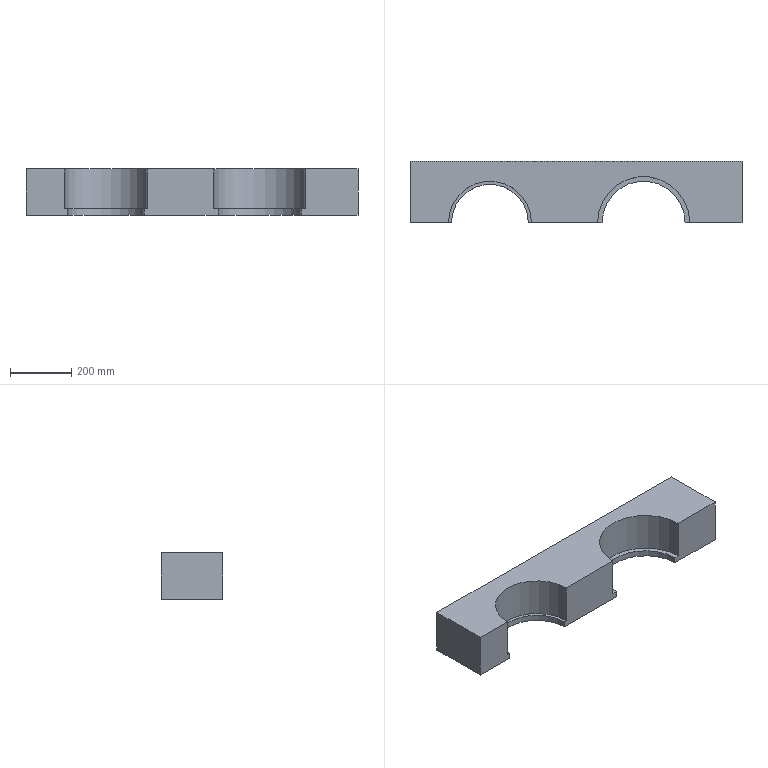Part | SolidWorks | features ICE 2, RefAxis 2, Extrusion 1 | 1 solid | 14 faces | box 1080 x 200 x 150 mm | volume 23020382 mm3 | plane 10 | cylinder 4 | commonest cylinder face diameters 270 x2 250 x1 300 x1
STEP:
#1=CARTESIAN_POINT('',(-540.,-100.,0.));
#2=VERTEX_POINT('',#1);
#3=CARTESIAN_POINT('',(-405.,-100.,0.));
#4=VERTEX_POINT('',#3);
#5=CARTESIAN_POINT('',(540.,-100.,0.));
#6=DIRECTION('',(1.,0.,0.));
#7=VECTOR('',#6,1000.);
#8=LINE('',#5,#7);
#9=EDGE_CURVE('',#2,#4,#8,.T.);
#10=ORIENTED_EDGE('',*,*,#9,.T.);
#11=CARTESIAN_POINT('',(-405.,-100.,20.));
#12=VERTEX_POINT('',#11);
#13=CARTESIAN_POINT('',(-405.,-100.,0.));
#14=DIRECTION('',(0.,0.,1.));
#15=VECTOR('',#14,1000.);
#16=LINE('',#13,#15);
#17=EDGE_CURVE('',#4,#12,#16,.T.);
#18=ORIENTED_EDGE('',*,*,#17,.T.);
#19=CARTESIAN_POINT('',(-415.,-100.,20.));
#20=VERTEX_POINT('',#19);
#21=CARTESIAN_POINT('',(540.,-100.,20.));
#22=DIRECTION('',(1.,0.,0.));
#23=VECTOR('',#22,1000.);
#24=LINE('',#21,#23);
#25=EDGE_CURVE('',#20,#12,#24,.T.);
#26=ORIENTED_EDGE('',*,*,#25,.F.);
#27=CARTESIAN_POINT('',(-415.,-100.,150.));
#28=VERTEX_POINT('',#27);
#29=CARTESIAN_POINT('',(-415.,-100.,20.));
#30=DIRECTION('',(0.,0.,1.));
#31=VECTOR('',#30,1000.);
#32=LINE('',#29,#31);
#33=EDGE_CURVE('',#20,#28,#32,.T.);
#34=ORIENTED_EDGE('',*,*,#33,.T.);
#35=CARTESIAN_POINT('',(-540.,-100.,150.));
#36=VERTEX_POINT('',#35);
#37=CARTESIAN_POINT('',(540.,-100.,150.));
#38=DIRECTION('',(1.,0.,0.));
#39=VECTOR('',#38,1000.);
#40=LINE('',#37,#39);
#41=EDGE_CURVE('',#36,#28,#40,.T.);
#42=ORIENTED_EDGE('',*,*,#41,.F.);
#43=CARTESIAN_POINT('',(-540.,-100.,150.));
#44=DIRECTION('',(0.,0.,-1.));
#45=VECTOR('',#44,1000.);
#46=LINE('',#43,#45);
#47=EDGE_CURVE('',#36,#2,#46,.T.);
#48=ORIENTED_EDGE('',*,*,#47,.T.);
#49=EDGE_LOOP('',(#10,#18,#26,#34,#42,#48));
#50=FACE_OUTER_BOUND('',#49,.T.);
#51=CARTESIAN_POINT('',(540.,-100.,150.));
#52=DIRECTION('',(0.,1.,0.));
#53=DIRECTION('',(-1.,0.,0.));
#54=AXIS2_PLACEMENT_3D('',#51,#52,#53);
#55=PLANE('',#54);
#56=ADVANCED_FACE('',(#50),#55,.F.);
#57=CARTESIAN_POINT('',(-155.,-100.,20.));
#58=VERTEX_POINT('',#57);
#59=CARTESIAN_POINT('',(-145.,-100.,20.));
#60=VERTEX_POINT('',#59);
#61=CARTESIAN_POINT('',(540.,-100.,20.));
#62=DIRECTION('',(1.,0.,0.));
#63=VECTOR('',#62,1000.);
#64=LINE('',#61,#63);
#65=EDGE_CURVE('',#58,#60,#64,.T.);
#66=ORIENTED_EDGE('',*,*,#65,.F.);
#67=CARTESIAN_POINT('',(-155.,-100.,0.));
#68=VERTEX_POINT('',#67);
#69=CARTESIAN_POINT('',(-155.,-100.,0.));
#70=DIRECTION('',(0.,0.,-1.));
#71=VECTOR('',#70,1000.);
#72=LINE('',#69,#71);
#73=EDGE_CURVE('',#58,#68,#72,.T.);
#74=ORIENTED_EDGE('',*,*,#73,.T.);
#75=CARTESIAN_POINT('',(85.,-100.,0.));
#76=VERTEX_POINT('',#75);
#77=CARTESIAN_POINT('',(540.,-100.,0.));
#78=DIRECTION('',(1.,0.,0.));
#79=VECTOR('',#78,1000.);
#80=LINE('',#77,#79);
#81=EDGE_CURVE('',#68,#76,#80,.T.);
#82=ORIENTED_EDGE('',*,*,#81,.T.);
#83=CARTESIAN_POINT('',(85.,-100.,20.));
#84=VERTEX_POINT('',#83);
#85=CARTESIAN_POINT('',(85.,-100.,0.));
#86=DIRECTION('',(0.,0.,1.));
#87=VECTOR('',#86,1000.);
#88=LINE('',#85,#87);
#89=EDGE_CURVE('',#76,#84,#88,.T.);
#90=ORIENTED_EDGE('',*,*,#89,.T.);
#91=CARTESIAN_POINT('',(70.,-100.,20.));
#92=VERTEX_POINT('',#91);
#93=CARTESIAN_POINT('',(540.,-100.,20.));
#94=DIRECTION('',(1.,0.,0.));
#95=VECTOR('',#94,1000.);
#96=LINE('',#93,#95);
#97=EDGE_CURVE('',#92,#84,#96,.T.);
#98=ORIENTED_EDGE('',*,*,#97,.F.);
#99=CARTESIAN_POINT('',(70.,-100.,150.));
#100=VERTEX_POINT('',#99);
#101=CARTESIAN_POINT('',(70.,-100.,20.));
#102=DIRECTION('',(0.,0.,1.));
#103=VECTOR('',#102,1000.);
#104=LINE('',#101,#103);
#105=EDGE_CURVE('',#92,#100,#104,.T.);
#106=ORIENTED_EDGE('',*,*,#105,.T.);
#107=CARTESIAN_POINT('',(-145.,-100.,150.));
#108=VERTEX_POINT('',#107);
#109=CARTESIAN_POINT('',(540.,-100.,150.));
#110=DIRECTION('',(1.,0.,0.));
#111=VECTOR('',#110,1000.);
#112=LINE('',#109,#111);
#113=EDGE_CURVE('',#108,#100,#112,.T.);
#114=ORIENTED_EDGE('',*,*,#113,.F.);
#115=CARTESIAN_POINT('',(-145.,-100.,20.));
#116=DIRECTION('',(0.,0.,-1.));
#117=VECTOR('',#116,1000.);
#118=LINE('',#115,#117);
#119=EDGE_CURVE('',#108,#60,#118,.T.);
#120=ORIENTED_EDGE('',*,*,#119,.T.);
#121=EDGE_LOOP('',(#66,#74,#82,#90,#98,#106,#114,#120));
#122=FACE_OUTER_BOUND('',#121,.T.);
#123=CARTESIAN_POINT('',(540.,-100.,150.));
#124=DIRECTION('',(0.,1.,0.));
#125=DIRECTION('',(-1.,0.,0.));
#126=AXIS2_PLACEMENT_3D('',#123,#124,#125);
#127=PLANE('',#126);
#128=ADVANCED_FACE('',(#122),#127,.F.);
#129=CARTESIAN_POINT('',(-540.,100.,0.));
#130=VERTEX_POINT('',#129);
#131=CARTESIAN_POINT('',(-540.,100.,0.));
#132=DIRECTION('',(0.,-1.,0.));
#133=VECTOR('',#132,1000.);
#134=LINE('',#131,#133);
#135=EDGE_CURVE('',#130,#2,#134,.T.);
#136=ORIENTED_EDGE('',*,*,#135,.T.);
#137=ORIENTED_EDGE('',*,*,#47,.F.);
#138=CARTESIAN_POINT('',(-540.,100.,150.));
#139=VERTEX_POINT('',#138);
#140=CARTESIAN_POINT('',(-540.,100.,150.));
#141=DIRECTION('',(0.,-1.,0.));
#142=VECTOR('',#141,1000.);
#143=LINE('',#140,#142);
#144=EDGE_CURVE('',#139,#36,#143,.T.);
#145=ORIENTED_EDGE('',*,*,#144,.F.);
#146=CARTESIAN_POINT('',(-540.,100.,150.));
#147=DIRECTION('',(0.,0.,-1.));
#148=VECTOR('',#147,1000.);
#149=LINE('',#146,#148);
#150=EDGE_CURVE('',#139,#130,#149,.T.);
#151=ORIENTED_EDGE('',*,*,#150,.T.);
#152=EDGE_LOOP('',(#136,#137,#145,#151));
#153=FACE_OUTER_BOUND('',#152,.T.);
#154=CARTESIAN_POINT('',(-540.,100.,150.));
#155=DIRECTION('',(1.,0.,0.));
#156=DIRECTION('',(0.,0.,-1.));
#157=AXIS2_PLACEMENT_3D('',#154,#155,#156);
#158=PLANE('',#157);
#159=ADVANCED_FACE('',(#153),#158,.F.);
#160=CARTESIAN_POINT('',(355.,-100.,20.));
#161=VERTEX_POINT('',#160);
#162=CARTESIAN_POINT('',(370.,-100.,20.));
#163=VERTEX_POINT('',#162);
#164=CARTESIAN_POINT('',(540.,-100.,20.));
#165=DIRECTION('',(1.,0.,0.));
#166=VECTOR('',#165,1000.);
#167=LINE('',#164,#166);
#168=EDGE_CURVE('',#161,#163,#167,.T.);
#169=ORIENTED_EDGE('',*,*,#168,.F.);
#170=CARTESIAN_POINT('',(355.,-100.,0.));
#171=VERTEX_POINT('',#170);
#172=CARTESIAN_POINT('',(355.,-100.,0.));
#173=DIRECTION('',(0.,0.,-1.));
#174=VECTOR('',#173,1000.);
#175=LINE('',#172,#174);
#176=EDGE_CURVE('',#161,#171,#175,.T.);
#177=ORIENTED_EDGE('',*,*,#176,.T.);
#178=CARTESIAN_POINT('',(540.,-100.,0.));
#179=VERTEX_POINT('',#178);
#180=CARTESIAN_POINT('',(540.,-100.,0.));
#181=DIRECTION('',(1.,0.,0.));
#182=VECTOR('',#181,1000.);
#183=LINE('',#180,#182);
#184=EDGE_CURVE('',#171,#179,#183,.T.);
#185=ORIENTED_EDGE('',*,*,#184,.T.);
#186=CARTESIAN_POINT('',(540.,-100.,150.));
#187=VERTEX_POINT('',#186);
#188=CARTESIAN_POINT('',(540.,-100.,150.));
#189=DIRECTION('',(0.,0.,-1.));
#190=VECTOR('',#189,1000.);
#191=LINE('',#188,#190);
#192=EDGE_CURVE('',#187,#179,#191,.T.);
#193=ORIENTED_EDGE('',*,*,#192,.F.);
#194=CARTESIAN_POINT('',(370.,-100.,150.));
#195=VERTEX_POINT('',#194);
#196=CARTESIAN_POINT('',(540.,-100.,150.));
#197=DIRECTION('',(1.,0.,0.));
#198=VECTOR('',#197,1000.);
#199=LINE('',#196,#198);
#200=EDGE_CURVE('',#195,#187,#199,.T.);
#201=ORIENTED_EDGE('',*,*,#200,.F.);
#202=CARTESIAN_POINT('',(370.,-100.,20.));
#203=DIRECTION('',(0.,0.,-1.));
#204=VECTOR('',#203,1000.);
#205=LINE('',#202,#204);
#206=EDGE_CURVE('',#195,#163,#205,.T.);
#207=ORIENTED_EDGE('',*,*,#206,.T.);
#208=EDGE_LOOP('',(#169,#177,#185,#193,#201,#207));
#209=FACE_OUTER_BOUND('',#208,.T.);
#210=CARTESIAN_POINT('',(540.,-100.,150.));
#211=DIRECTION('',(0.,1.,0.));
#212=DIRECTION('',(-1.,0.,0.));
#213=AXIS2_PLACEMENT_3D('',#210,#211,#212);
#214=PLANE('',#213);
#215=ADVANCED_FACE('',(#209),#214,.F.);
#216=CARTESIAN_POINT('',(540.,100.,0.));
#217=VERTEX_POINT('',#216);
#218=CARTESIAN_POINT('',(540.,100.,0.));
#219=DIRECTION('',(0.,1.,0.));
#220=VECTOR('',#219,1000.);
#221=LINE('',#218,#220);
#222=EDGE_CURVE('',#179,#217,#221,.T.);
#223=ORIENTED_EDGE('',*,*,#222,.T.);
#224=CARTESIAN_POINT('',(540.,100.,150.));
#225=VERTEX_POINT('',#224);
#226=CARTESIAN_POINT('',(540.,100.,150.));
#227=DIRECTION('',(0.,0.,-1.));
#228=VECTOR('',#227,1000.);
#229=LINE('',#226,#228);
#230=EDGE_CURVE('',#225,#217,#229,.T.);
#231=ORIENTED_EDGE('',*,*,#230,.F.);
#232=CARTESIAN_POINT('',(540.,100.,150.));
#233=DIRECTION('',(0.,1.,0.));
#234=VECTOR('',#233,1000.);
#235=LINE('',#232,#234);
#236=EDGE_CURVE('',#187,#225,#235,.T.);
#237=ORIENTED_EDGE('',*,*,#236,.F.);
#238=ORIENTED_EDGE('',*,*,#192,.T.);
#239=EDGE_LOOP('',(#223,#231,#237,#238));
#240=FACE_OUTER_BOUND('',#239,.T.);
#241=CARTESIAN_POINT('',(540.,100.,150.));
#242=DIRECTION('',(-1.,0.,0.));
#243=DIRECTION('',(0.,-1.,0.));
#244=AXIS2_PLACEMENT_3D('',#241,#242,#243);
#245=PLANE('',#244);
#246=ADVANCED_FACE('',(#240),#245,.F.);
#247=CARTESIAN_POINT('',(540.,100.,0.));
#248=DIRECTION('',(-1.,0.,0.));
#249=VECTOR('',#248,1000.);
#250=LINE('',#247,#249);
#251=EDGE_CURVE('',#217,#130,#250,.T.);
#252=ORIENTED_EDGE('',*,*,#251,.T.);
#253=ORIENTED_EDGE('',*,*,#150,.F.);
#254=CARTESIAN_POINT('',(540.,100.,150.));
#255=DIRECTION('',(-1.,0.,0.));
#256=VECTOR('',#255,1000.);
#257=LINE('',#254,#256);
#258=EDGE_CURVE('',#225,#139,#257,.T.);
#259=ORIENTED_EDGE('',*,*,#258,.F.);
#260=ORIENTED_EDGE('',*,*,#230,.T.);
#261=EDGE_LOOP('',(#252,#253,#259,#260));
#262=FACE_OUTER_BOUND('',#261,.T.);
#263=CARTESIAN_POINT('',(540.,100.,150.));
#264=DIRECTION('',(0.,-1.,0.));
#265=DIRECTION('',(1.,0.,0.));
#266=AXIS2_PLACEMENT_3D('',#263,#264,#265);
#267=PLANE('',#266);
#268=ADVANCED_FACE('',(#262),#267,.F.);
#269=ORIENTED_EDGE('',*,*,#41,.T.);
#270=CARTESIAN_POINT('',(-280.,-100.,150.));
#271=DIRECTION('',(0.,0.,1.));
#272=DIRECTION('',(1.,0.,0.));
#273=AXIS2_PLACEMENT_3D('',#270,#271,#272);
#274=CIRCLE('',#273,135.);
#275=EDGE_CURVE('',#108,#28,#274,.T.);
#276=ORIENTED_EDGE('',*,*,#275,.F.);
#277=ORIENTED_EDGE('',*,*,#113,.T.);
#278=CARTESIAN_POINT('',(220.,-100.,150.));
#279=DIRECTION('',(0.,0.,1.));
#280=DIRECTION('',(1.,0.,0.));
#281=AXIS2_PLACEMENT_3D('',#278,#279,#280);
#282=CIRCLE('',#281,150.);
#283=EDGE_CURVE('',#195,#100,#282,.T.);
#284=ORIENTED_EDGE('',*,*,#283,.F.);
#285=ORIENTED_EDGE('',*,*,#200,.T.);
#286=ORIENTED_EDGE('',*,*,#236,.T.);
#287=ORIENTED_EDGE('',*,*,#258,.T.);
#288=ORIENTED_EDGE('',*,*,#144,.T.);
#289=EDGE_LOOP('',(#269,#276,#277,#284,#285,#286,#287,#288));
#290=FACE_OUTER_BOUND('',#289,.T.);
#291=CARTESIAN_POINT('',(0.,0.,150.));
#292=DIRECTION('',(0.,0.,-1.));
#293=DIRECTION('',(-1.,0.,0.));
#294=AXIS2_PLACEMENT_3D('',#291,#292,#293);
#295=PLANE('',#294);
#296=ADVANCED_FACE('',(#290),#295,.F.);
#297=CARTESIAN_POINT('',(-280.,-100.,0.));
#298=DIRECTION('',(0.,0.,1.));
#299=DIRECTION('',(1.,0.,0.));
#300=AXIS2_PLACEMENT_3D('',#297,#298,#299);
#301=CIRCLE('',#300,125.);
#302=EDGE_CURVE('',#68,#4,#301,.T.);
#303=ORIENTED_EDGE('',*,*,#302,.T.);
#304=ORIENTED_EDGE('',*,*,#9,.F.);
#305=ORIENTED_EDGE('',*,*,#135,.F.);
#306=ORIENTED_EDGE('',*,*,#251,.F.);
#307=ORIENTED_EDGE('',*,*,#222,.F.);
#308=ORIENTED_EDGE('',*,*,#184,.F.);
#309=CARTESIAN_POINT('',(220.,-100.,0.));
#310=DIRECTION('',(0.,0.,1.));
#311=DIRECTION('',(1.,0.,0.));
#312=AXIS2_PLACEMENT_3D('',#309,#310,#311);
#313=CIRCLE('',#312,135.);
#314=EDGE_CURVE('',#171,#76,#313,.T.);
#315=ORIENTED_EDGE('',*,*,#314,.T.);
#316=ORIENTED_EDGE('',*,*,#81,.F.);
#317=EDGE_LOOP('',(#303,#304,#305,#306,#307,#308,#315,#316));
#318=FACE_OUTER_BOUND('',#317,.T.);
#319=CARTESIAN_POINT('',(0.,0.,0.));
#320=DIRECTION('',(0.,0.,-1.));
#321=DIRECTION('',(-1.,0.,0.));
#322=AXIS2_PLACEMENT_3D('',#319,#320,#321);
#323=PLANE('',#322);
#324=ADVANCED_FACE('',(#318),#323,.T.);
#325=CARTESIAN_POINT('',(220.,-100.,20.));
#326=DIRECTION('',(0.,0.,1.));
#327=DIRECTION('',(1.,0.,0.));
#328=AXIS2_PLACEMENT_3D('',#325,#326,#327);
#329=CIRCLE('',#328,135.);
#330=EDGE_CURVE('',#161,#84,#329,.T.);
#331=ORIENTED_EDGE('',*,*,#330,.F.);
#332=ORIENTED_EDGE('',*,*,#168,.T.);
#333=CARTESIAN_POINT('',(220.,-100.,20.));
#334=DIRECTION('',(0.,0.,1.));
#335=DIRECTION('',(1.,0.,0.));
#336=AXIS2_PLACEMENT_3D('',#333,#334,#335);
#337=CIRCLE('',#336,150.);
#338=EDGE_CURVE('',#163,#92,#337,.T.);
#339=ORIENTED_EDGE('',*,*,#338,.T.);
#340=ORIENTED_EDGE('',*,*,#97,.T.);
#341=EDGE_LOOP('',(#331,#332,#339,#340));
#342=FACE_OUTER_BOUND('',#341,.T.);
#343=CARTESIAN_POINT('',(220.,-100.,20.));
#344=DIRECTION('',(0.,0.,1.));
#345=DIRECTION('',(1.,0.,0.));
#346=AXIS2_PLACEMENT_3D('',#343,#344,#345);
#347=PLANE('',#346);
#348=ADVANCED_FACE('',(#342),#347,.T.);
#349=ORIENTED_EDGE('',*,*,#338,.F.);
#350=ORIENTED_EDGE('',*,*,#206,.F.);
#351=ORIENTED_EDGE('',*,*,#283,.T.);
#352=ORIENTED_EDGE('',*,*,#105,.F.);
#353=EDGE_LOOP('',(#349,#350,#351,#352));
#354=FACE_OUTER_BOUND('',#353,.T.);
#355=CARTESIAN_POINT('',(220.,-100.,20.));
#356=DIRECTION('',(0.,0.,1.));
#357=DIRECTION('',(1.,0.,0.));
#358=AXIS2_PLACEMENT_3D('',#355,#356,#357);
#359=CYLINDRICAL_SURFACE('',#358,150.);
#360=ADVANCED_FACE('',(#354),#359,.F.);
#361=CARTESIAN_POINT('',(-280.,-100.,20.));
#362=DIRECTION('',(0.,0.,1.));
#363=DIRECTION('',(1.,0.,0.));
#364=AXIS2_PLACEMENT_3D('',#361,#362,#363);
#365=CIRCLE('',#364,125.);
#366=EDGE_CURVE('',#58,#12,#365,.T.);
#367=ORIENTED_EDGE('',*,*,#366,.F.);
#368=ORIENTED_EDGE('',*,*,#65,.T.);
#369=CARTESIAN_POINT('',(-280.,-100.,20.));
#370=DIRECTION('',(0.,0.,1.));
#371=DIRECTION('',(1.,0.,0.));
#372=AXIS2_PLACEMENT_3D('',#369,#370,#371);
#373=CIRCLE('',#372,135.);
#374=EDGE_CURVE('',#60,#20,#373,.T.);
#375=ORIENTED_EDGE('',*,*,#374,.T.);
#376=ORIENTED_EDGE('',*,*,#25,.T.);
#377=EDGE_LOOP('',(#367,#368,#375,#376));
#378=FACE_OUTER_BOUND('',#377,.T.);
#379=CARTESIAN_POINT('',(-280.,-100.,20.));
#380=DIRECTION('',(0.,0.,1.));
#381=DIRECTION('',(1.,0.,0.));
#382=AXIS2_PLACEMENT_3D('',#379,#380,#381);
#383=PLANE('',#382);
#384=ADVANCED_FACE('',(#378),#383,.T.);
#385=ORIENTED_EDGE('',*,*,#374,.F.);
#386=ORIENTED_EDGE('',*,*,#119,.F.);
#387=ORIENTED_EDGE('',*,*,#275,.T.);
#388=ORIENTED_EDGE('',*,*,#33,.F.);
#389=EDGE_LOOP('',(#385,#386,#387,#388));
#390=FACE_OUTER_BOUND('',#389,.T.);
#391=CARTESIAN_POINT('',(-280.,-100.,20.));
#392=DIRECTION('',(0.,0.,1.));
#393=DIRECTION('',(1.,0.,0.));
#394=AXIS2_PLACEMENT_3D('',#391,#392,#393);
#395=CYLINDRICAL_SURFACE('',#394,135.);
#396=ADVANCED_FACE('',(#390),#395,.F.);
#397=ORIENTED_EDGE('',*,*,#302,.F.);
#398=ORIENTED_EDGE('',*,*,#73,.F.);
#399=ORIENTED_EDGE('',*,*,#366,.T.);
#400=ORIENTED_EDGE('',*,*,#17,.F.);
#401=EDGE_LOOP('',(#397,#398,#399,#400));
#402=FACE_OUTER_BOUND('',#401,.T.);
#403=CARTESIAN_POINT('',(-280.,-100.,0.));
#404=DIRECTION('',(0.,0.,1.));
#405=DIRECTION('',(1.,0.,0.));
#406=AXIS2_PLACEMENT_3D('',#403,#404,#405);
#407=CYLINDRICAL_SURFACE('',#406,125.);
#408=ADVANCED_FACE('',(#402),#407,.F.);
#409=ORIENTED_EDGE('',*,*,#314,.F.);
#410=ORIENTED_EDGE('',*,*,#176,.F.);
#411=ORIENTED_EDGE('',*,*,#330,.T.);
#412=ORIENTED_EDGE('',*,*,#89,.F.);
#413=EDGE_LOOP('',(#409,#410,#411,#412));
#414=FACE_OUTER_BOUND('',#413,.T.);
#415=CARTESIAN_POINT('',(220.,-100.,0.));
#416=DIRECTION('',(0.,0.,1.));
#417=DIRECTION('',(1.,0.,0.));
#418=AXIS2_PLACEMENT_3D('',#415,#416,#417);
#419=CYLINDRICAL_SURFACE('',#418,135.);
#420=ADVANCED_FACE('',(#414),#419,.F.);
#421=CLOSED_SHELL('',(#56,#128,#159,#215,#246,#268,#296,#324,#348,#360,#384,#396,#408,#420));
#422=MANIFOLD_SOLID_BREP('',#421);
#423=CARTESIAN_POINT('',(0.,0.,0.));
#424=DIRECTION('',(0.,0.,1.));
#425=DIRECTION('',(1.,0.,0.));
#426=AXIS2_PLACEMENT_3D('',#423,#424,#425);
#427=(LENGTH_UNIT()NAMED_UNIT(*)SI_UNIT(.MILLI.,.METRE.));
#428=UNCERTAINTY_MEASURE_WITH_UNIT(LENGTH_MEASURE(0.00001),#427,'','');
#429=(NAMED_UNIT(*)PLANE_ANGLE_UNIT()SI_UNIT($,.RADIAN.));
#430=(NAMED_UNIT(*)SI_UNIT($,.STERADIAN.)SOLID_ANGLE_UNIT());
#431=(GEOMETRIC_REPRESENTATION_CONTEXT(3)GLOBAL_UNCERTAINTY_ASSIGNED_CONTEXT((#428))GLOBAL_UNIT_ASSIGNED_CONTEXT((#427,#429,#430))REPRESENTATION_CONTEXT('',''));
#432=ADVANCED_BREP_SHAPE_REPRESENTATION('',(#422,#426),#431);